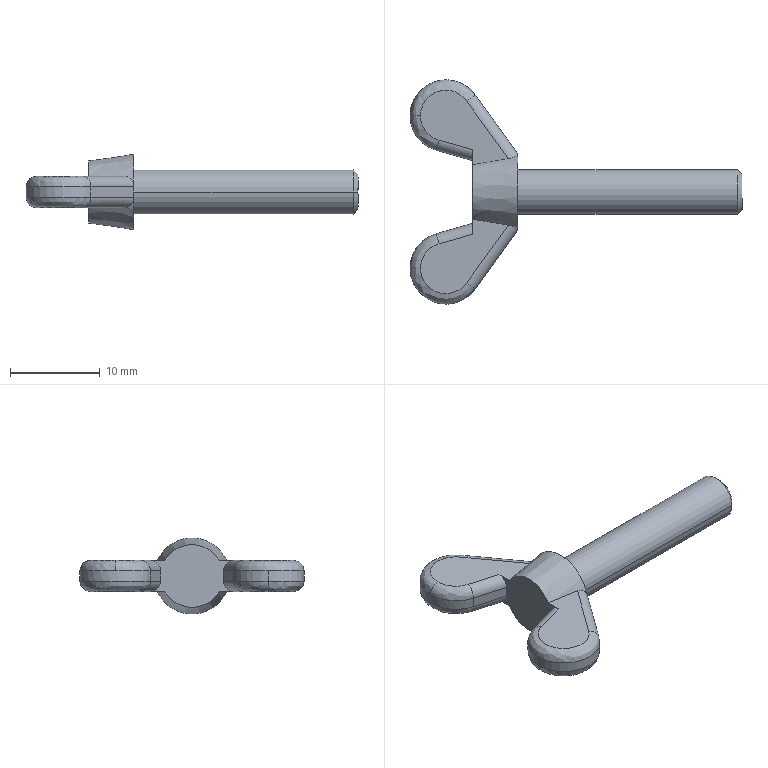Part | STEP file | JIS B 1184 - M5 x 25 | 1 solid | 34 faces | box 37 x 25 x 8.5 mm | volume 1182 mm3 | cylinder 13 | plane 11 | spline 6 | cone 4 | commonest cylinder face diameters 2.333 x8 8 x3 5 x2